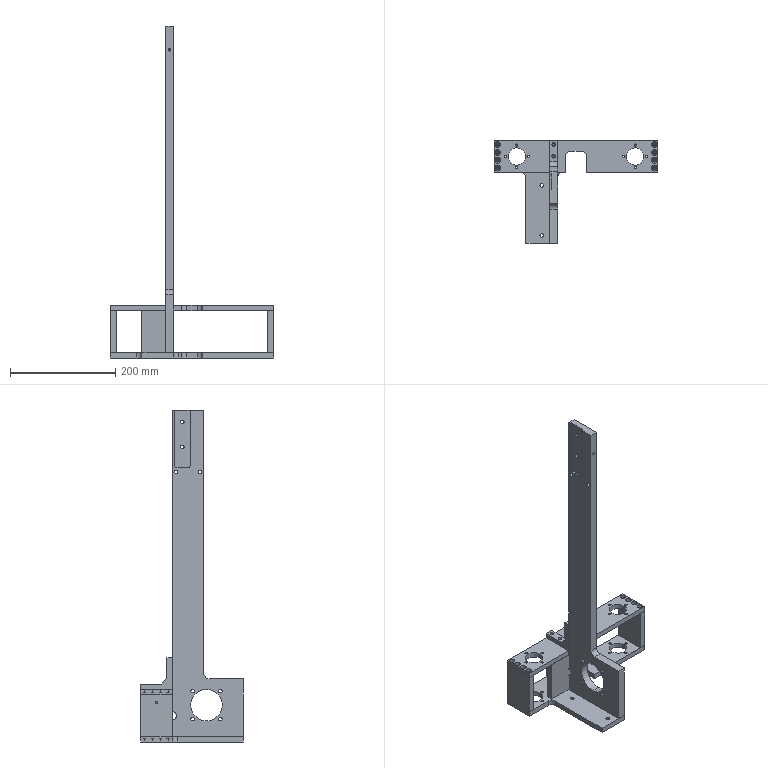Part | STEP file | Lifting frame_default<machined> | 7 solids | 411 faces | box 310 x 195 x 630 mm | volume 1240062 mm3 | cylinder 257 | plane 98 | cone 56 | commonest cylinder face diameters 5 x64 6.6 x58 11 x50 4.2 x32 6.8 x16 6.5 x8